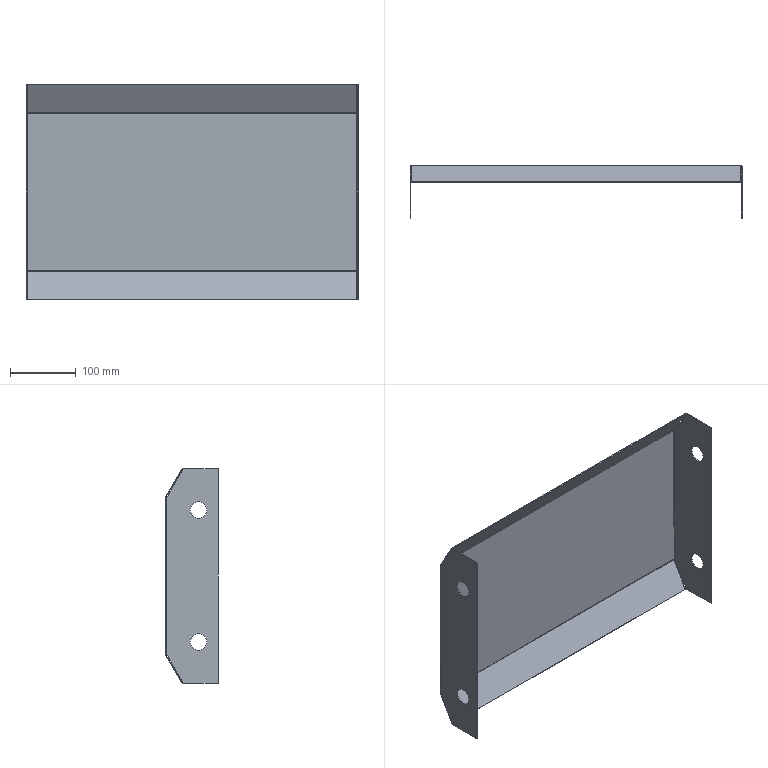Part | STEP file | 1 solid | 50 faces | box 504 x 80 x 327.138 mm | volume 217824 mm3 | plane 34 | cylinder 16 | commonest cylinder face diameters 25.2 x8 2 x4 4 x4